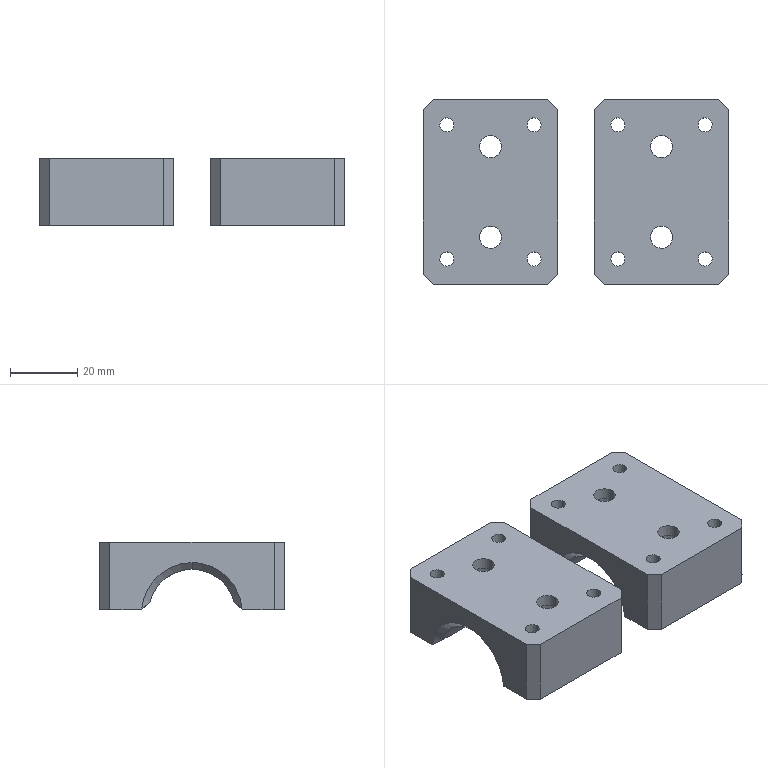NC program | NX | posted with a generic post | part box 91 x 55 x 20 mm
Whole program:
N10 G17 G21 G94 G90
(FLOOR_WALL_COPY_COPY , TOOL : D80)
N12 T19 M6
N14 G54
N16 G17 G0 G90 X90.5 Y0. S6500 M3
N18 G43 Z30. H19
N20 Z7.
N22 G94 G1 Z4. F1500.
N24 X85.5
N26 X-85.5
N28 X-90.5
N30 Z7.
N32 G0 Z30.
N34 X90.5
N36 Z6.
N38 G1 Z3.
N40 X85.5
N42 X-85.5
N44 X-90.5
N46 Z6.
N48 G0 Z30.
N50 X90.5
N52 Z5.
N54 G1 Z2.
N56 X85.5
N58 X-85.5
N60 X-90.5
N62 Z5.
N64 G0 Z30.
N66 X90.5
N68 Z4.
N70 G1 Z1.
N72 X85.5
N74 X-85.5
N76 X-90.5
N78 Z4.
N80 G0 Z30.
N82 X90.5
N84 Z3.
N86 G1 Z0.
N88 X85.5
N90 X-85.5
N92 X-90.5
N94 Z3.
N96 G0 Z30.
N98 M5
(PLANAR_MILL_COPY_COPY_COPY_COPY_COPY_COPY_1_1 , TOOL : D6A45)
N100 T01 M6
N102 G54
N104 G17 G0 G90 X13.365 Y20.698 S9500 M3
N106 G43 Z30. H1
N108 Z0.5
N110 G94 G1 Z-1. F1250.
N112 G3 X12.499 Y21.198 R1.
N114 X11.792 Y20.969 R1.207
N116 X11.431 Y20.547 R1.179
N118 X11.431 Y19.453 R1.209
N120 X11.792 Y19.031 R1.179
N122 X13.046 Y18.933 R1.207
N124 X13.046 Y21.067 R1.197
N126 X12.499 Y21.198 R1.207
N128 X11.633 Y20.698 R1.
N130 G1 Z0.5
N132 G0 Z30.
N134 X26.364 Y15.397
N136 Z0.5
N138 G1 Z-1.
N140 G3 X25.498 Y15.897 R1.
N142 X24.086 Y15.44 R2.411
N144 X23.361 Y14.592 R2.367
N146 X23.361 Y12.408 R2.414
N148 X24.086 Y11.56 R2.367
N150 X26.591 Y11.365 R2.411
N152 X26.591 Y15.635 R2.395
N154 X25.498 Y15.897 R2.411
N156 X24.632 Y15.397 R1.
N158 G1 Z0.5
N160 G0 Z30.
N162 X39.2 Y19.134
N164 Z0.5
N166 G1 Z-1.
N168 G3 X39.7 Y20. R1.
N170 X39.046 Y21.067 R1.197
N172 X37.792 Y20.969 R1.207
N174 X37.431 Y20.547 R1.179
N176 X37.431 Y19.453 R1.209
N178 X37.792 Y19.031 R1.179
N180 X39.046 Y18.933 R1.207
N182 X39.7 Y20. R1.197
N184 X39.2 Y20.866 R1.
N186 G1 Z0.5
N188 G0 Z30.
N190 X46.9 Y0.866
N192 Z0.5
N194 G1 Z-1.
N196 G3 X46.4 Y0. R1.
N198 G1 Y-24.5
N200 G2 X46.136 Y-25.136 R0.9
N202 G1 X43.136 Y-28.136
N204 G2 X42.5 Y-28.4 R0.9
N206 G1 X8.5
N208 G2 X7.864 Y-28.136 R0.9
N210 G1 X4.864 Y-25.136
N212 G2 X4.6 Y-24.5 R0.9
N214 G1 Y24.5
N216 G2 X4.864 Y25.136 R0.9
N218 G1 X7.864 Y28.136
N220 G2 X8.5 Y28.4 R0.9
N222 G1 X42.5
N224 G2 X43.136 Y28.136 R0.9
N226 G1 X46.136 Y25.136
N228 G2 X46.4 Y24.5 R0.9
N230 G1 Y0.
N232 G3 X46.9 Y-0.866 R1.
N234 G1 Z0.5
N236 G0 Z30.
N238 X39.2 Y-20.866
N240 Z0.5
N242 G1 Z-1.
N244 G3 X39.7 Y-20. R1.
N246 X39.046 Y-18.933 R1.197
N248 X37.792 Y-19.031 R1.207
N250 X37.431 Y-19.453 R1.179
N252 X37.431 Y-20.547 R1.209
N254 X37.792 Y-20.969 R1.179
N256 X39.046 Y-21.067 R1.207
N258 X39.7 Y-20. R1.197
N260 X39.2 Y-19.134 R1.
N262 G1 Z0.5
N264 G0 Z30.
N266 X24.632 Y-15.397
N268 Z0.5
N270 G1 Z-1.
N272 G3 X25.498 Y-15.897 R1.
N274 X26.591 Y-15.635 R2.411
N276 X26.591 Y-11.365 R2.395
N278 X24.086 Y-11.56 R2.411
N280 X23.361 Y-12.408 R2.367
N282 X23.361 Y-14.592 R2.414
N284 X24.086 Y-15.44 R2.367
N286 X25.498 Y-15.897 R2.411
N288 X26.364 Y-15.397 R1.
N290 G1 Z0.5
N292 G0 Z30.
N294 X11.633 Y-20.698
N296 Z0.5
N298 G1 Z-1.
N300 G3 X12.499 Y-21.198 R1.
N302 X13.046 Y-21.067 R1.207
N304 X13.046 Y-18.933 R1.197
N306 X11.792 Y-19.031 R1.207
N308 X11.431 Y-19.453 R1.179
N310 X11.431 Y-20.547 R1.209
N312 X11.792 Y-20.969 R1.179
N314 X12.499 Y-21.198 R1.207
N316 X13.365 Y-20.698 R1.
N318 G1 Z0.5
N320 G0 Z30.
N322 X-13.367
N324 Z0.5
N326 G1 Z-1.
N328 G3 X-12.501 Y-21.198 R1.
N330 X-11.954 Y-21.067 R1.207
N332 X-11.954 Y-18.933 R1.197
N334 X-13.208 Y-19.031 R1.207
N336 X-13.569 Y-19.453 R1.179
N338 X-13.569 Y-20.547 R1.209
N340 X-13.208 Y-20.969 R1.179
N342 X-12.501 Y-21.198 R1.207
N344 X-11.635 Y-20.698 R1.
N346 G1 Z0.5
N348 G0 Z30.
N350 X-26.368 Y-15.397
N352 Z0.5
N354 G1 Z-1.
N356 G3 X-25.502 Y-15.897 R1.
N358 X-24.409 Y-15.635 R2.411
N360 X-24.409 Y-11.365 R2.395
N362 X-26.914 Y-11.56 R2.411
N364 X-27.639 Y-12.408 R2.367
N366 X-27.639 Y-14.592 R2.414
N368 X-26.914 Y-15.44 R2.367
N370 X-25.502 Y-15.897 R2.411
N372 X-24.636 Y-15.397 R1.
N374 G1 Z0.5
N376 G0 Z30.
N378 X-39.2 Y-19.134
N380 Z0.5
N382 G1 Z-1.
N384 G3 X-39.7 Y-20. R1.
N386 X-39.046 Y-21.067 R1.197
N388 X-37.792 Y-20.969 R1.207
N390 X-37.431 Y-20.547 R1.179
N392 X-37.431 Y-19.453 R1.209
N394 X-37.792 Y-19.031 R1.179
N396 X-39.046 Y-18.933 R1.207
N398 X-39.7 Y-20. R1.197
N400 X-39.2 Y-20.866 R1.
N402 G1 Z0.5
N404 G0 Z30.
N406 X-46.9 Y-0.866
N408 Z0.5
N410 G1 Z-1.
N412 G3 X-46.4 Y0. R1.
N414 G1 Y24.5
N416 G2 X-46.136 Y25.136 R0.9
N418 G1 X-43.136 Y28.136
N420 G2 X-42.5 Y28.4 R0.9
N422 G1 X-8.5
N424 G2 X-7.864 Y28.136 R0.9
N426 G1 X-4.864 Y25.136
N428 G2 X-4.6 Y24.5 R0.9
N430 G1 Y-24.5
N432 G2 X-4.864 Y-25.136 R0.9
N434 G1 X-7.864 Y-28.136
N436 G2 X-8.5 Y-28.4 R0.9
N438 G1 X-42.5
N440 G2 X-43.136 Y-28.136 R0.9
N442 G1 X-46.136 Y-25.136
N444 G2 X-46.4 Y-24.5 R0.9
N446 G1 Y0.
N448 G3 X-46.9 Y0.866 R1.
N450 G1 Z0.5
N452 G0 Z30.
N454 X-11.635 Y20.698
N456 Z0.5
N458 G1 Z-1.
N460 G3 X-12.501 Y21.198 R1.
N462 X-13.208 Y20.969 R1.207
N464 X-13.569 Y20.547 R1.179
N466 X-13.569 Y19.453 R1.209
N468 X-13.208 Y19.031 R1.179
N470 X-11.954 Y18.933 R1.207
N472 X-11.954 Y21.067 R1.197
N474 X-12.501 Y21.198 R1.207
N476 X-13.367 Y20.698 R1.
N478 G1 Z0.5
N480 G0 Z30.
N482 X-24.632 Y15.397
N484 Z0.5
N486 G1 Z-1.
N488 G3 X-25.498 Y15.897 R1.
N490 X-26.591 Y15.635 R2.411
N492 X-26.591 Y11.365 R2.395
N494 X-24.086 Y11.56 R2.411
N496 X-23.361 Y12.408 R2.367
N498 X-23.361 Y14.592 R2.414
N500 X-24.086 Y15.44 R2.367
N502 X-25.498 Y15.897 R2.411
N504 X-26.364 Y15.397 R1.
N506 G1 Z0.5
N508 G0 Z30.
N510 X-39.2 Y20.866
N512 Z0.5
N514 G1 Z-1.
N516 G3 X-39.7 Y20. R1.
N518 X-39.046 Y18.933 R1.197
N520 X-37.792 Y19.031 R1.207
N522 X-37.431 Y19.453 R1.179
N524 X-37.431 Y20.547 R1.209
N526 X-37.792 Y20.969 R1.179
N528 X-39.046 Y21.067 R1.207
N530 X-39.7 Y20. R1.197
N532 X-39.2 Y19.134 R1.
N534 G1 Z0.5
N536 G0 Z30.
N538 M5
N540 M2